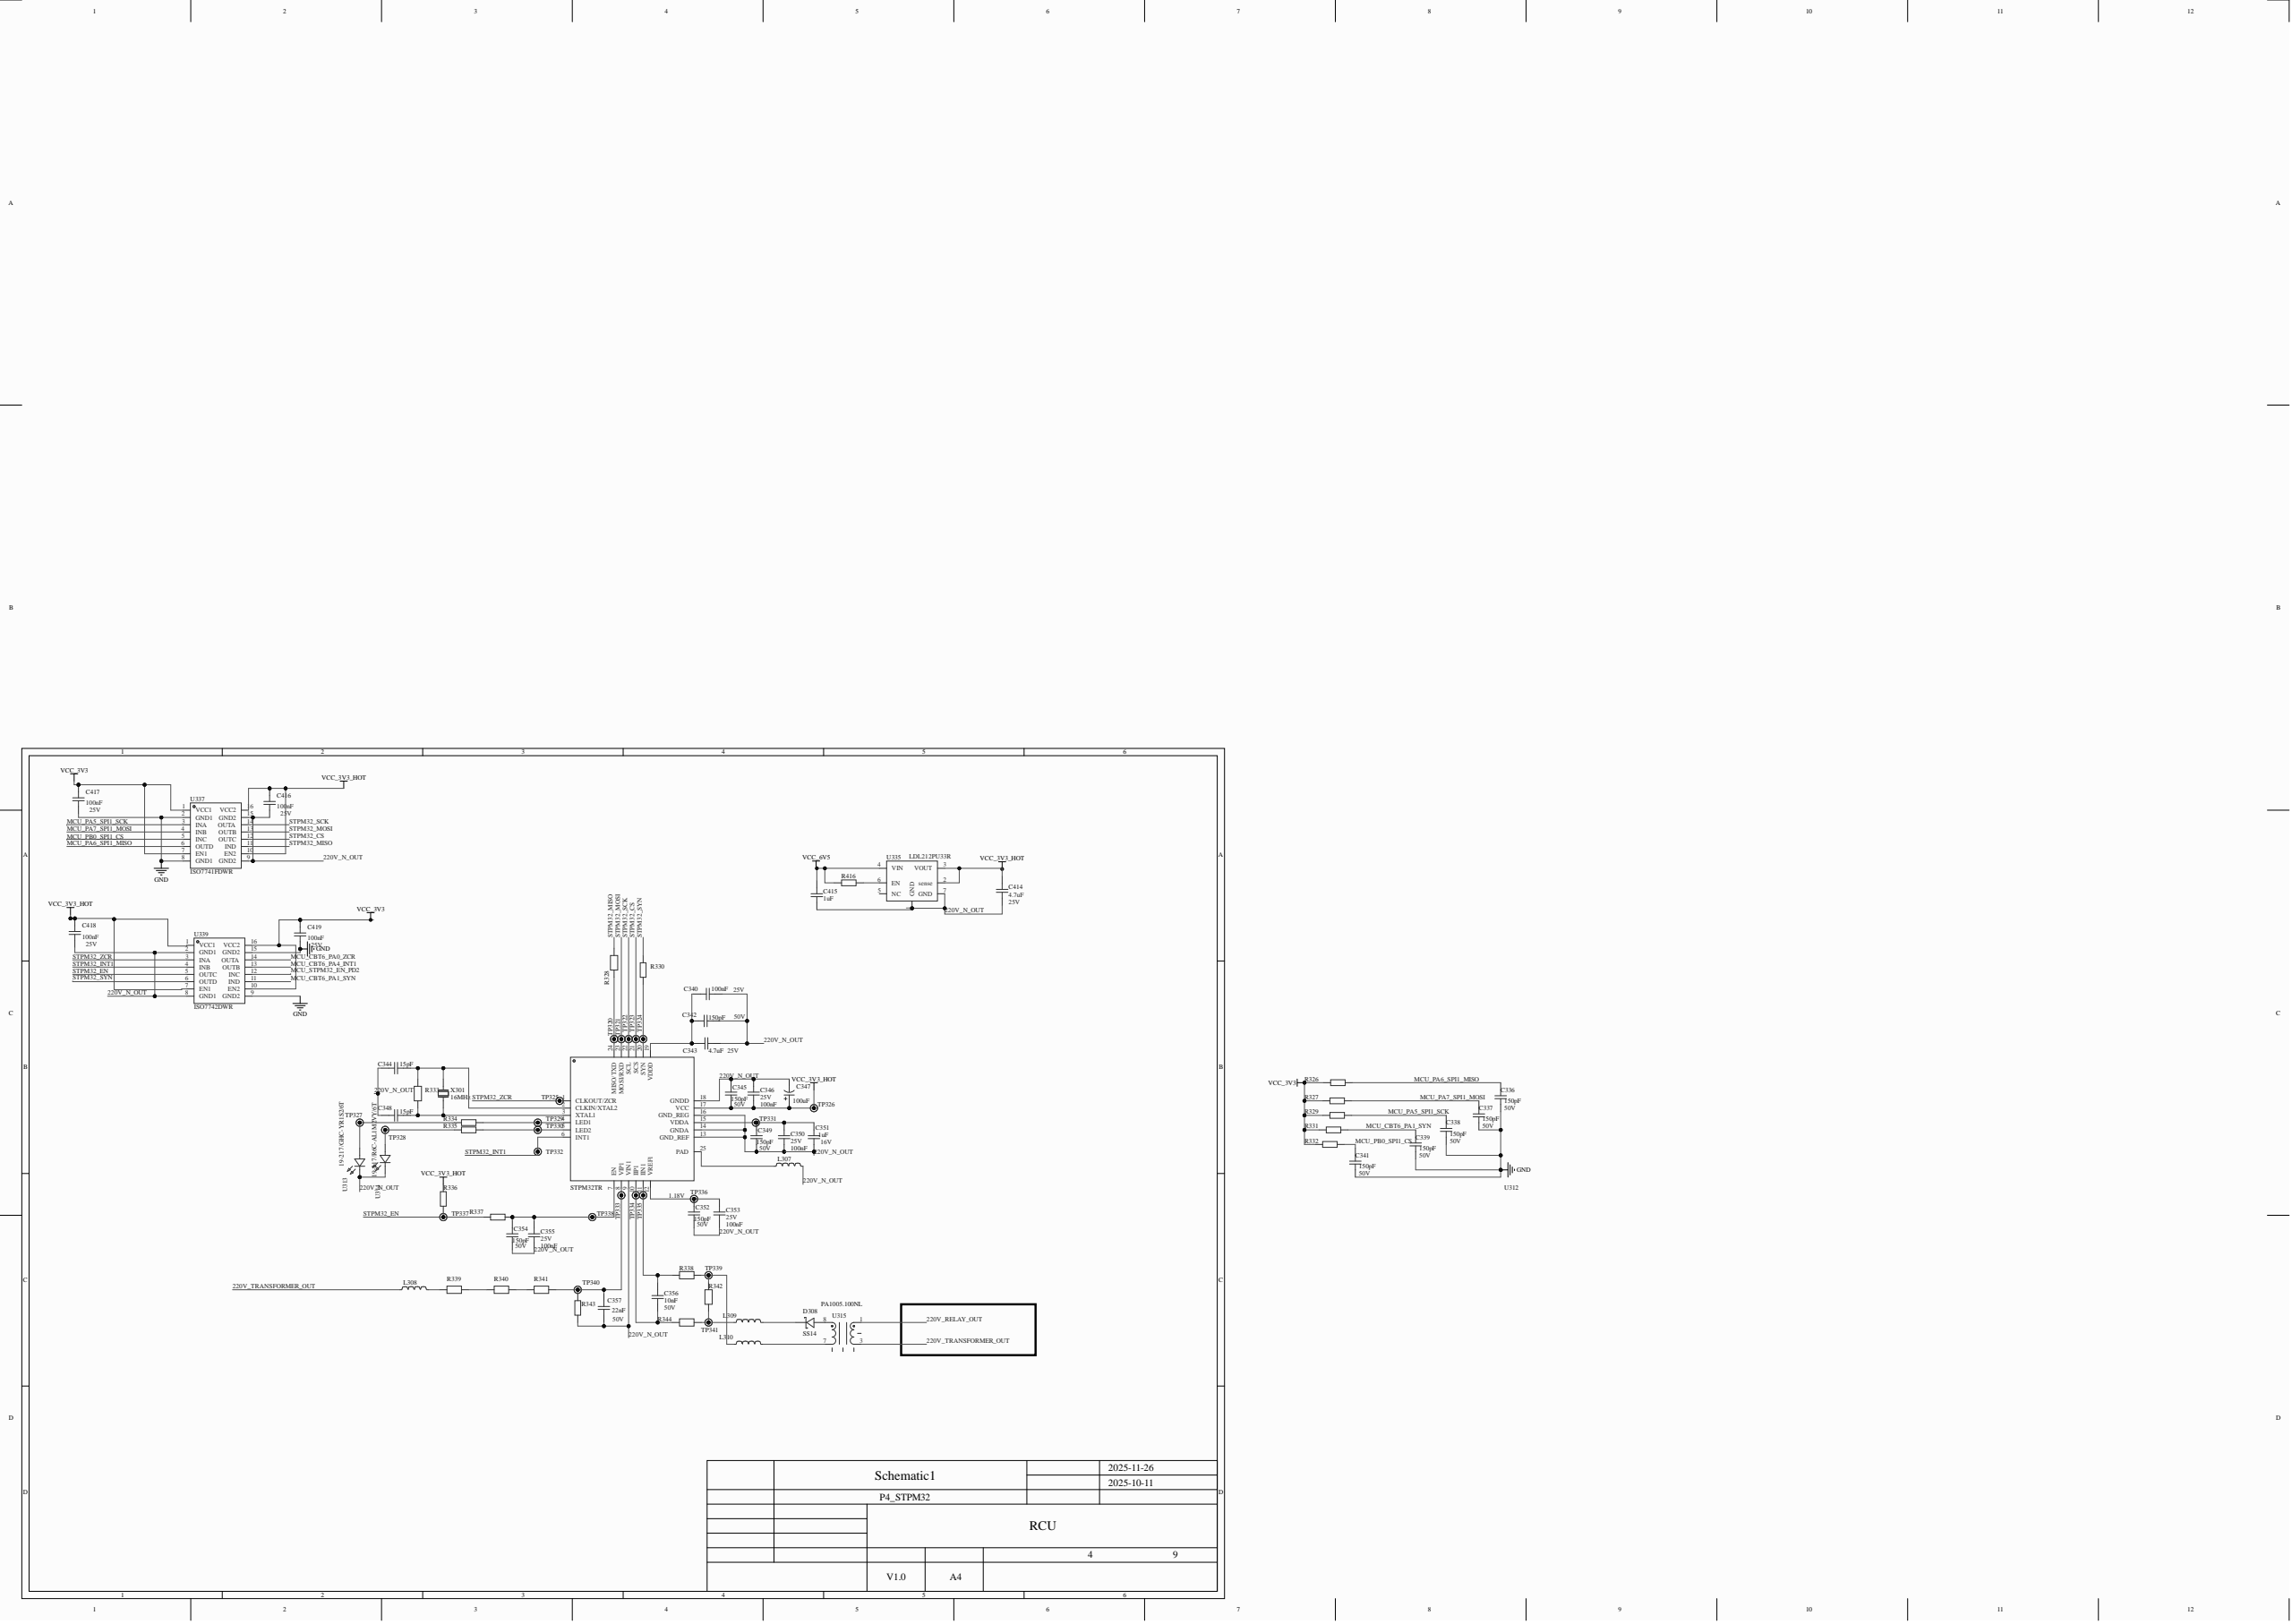Circuit board | Altium Designer | 424 parts | 202 nets | one sheet of the schematic
Parts on this sheet (reference | value | footprint):
C336 | 150pF | C0603
C337 | 150pF | C0603
C338 | 150pF | C0603
C339 | 150pF | C0603
C340 | 100nF | C0603
C341 | 150pF | C0603
C342 | 150pF | C0603
C343 | 4.7uF | C0603
C344 | 15pF | C0603
C345 | 150pF | C0603
C346 | 100nF | C0603
C347 | 100uF | CAP-SMD_BD6.3-L6.6-W6.6-LS7.3-FD-H7.7
C348 | 15pF | C0603
C349 | 150pF | C0603
C350 | 100nF | C0603
C351 | 1uF | C0603
C352 | 150pF | C0603
C353 | 100nF | C0603
C354 | 150pF | C0603
C355 | 100nF | C0603
C356 | 10nF | C0603
C357 | 22nF | C0805
C414 | 4.7uF | C0603
C415 | 1uF | C0603
C416 | 100nF | C0603
C417 | 100nF | C0603
C418 | 100nF | C0603
C419 | 100nF | C0603
D308 | SS14 | SMA_L4.3-W2.6-LS5.2-RD
L307 | L0805
L308 | L0805
L309 | L0805
L310 | L0805
R326 | R0603
R327 | R0603
R328 | R0603
R329 | R0603
R330 | R0603
R331 | R0603
R332 | R0603
R333 | R0603
R334 | R0603
R335 | R0603
R336 | R0603
R337 | R0603
R338 | R1206
R339 | R1206
R340 | R1206
R341 | R1206
R342 | R1206
R343 | R1206
R344 | R1206
R416 | R0603
TP320 | Test-Point-0.5mm
TP321 | Test-Point-0.5mm
TP322 | Test-Point-0.5mm
TP323 | Test-Point-0.5mm
TP324 | Test-Point-0.5mm
TP325 | Test-Point-0.5mm
TP326 | Test-Point-0.5mm
TP327 | Test-Point-0.5mm
TP328 | Test-Point-0.5mm
TP329 | Test-Point-0.5mm
TP330 | Test-Point-0.5mm
TP331 | Test-Point-0.5mm
TP332 | Test-Point-0.5mm
TP333 | Test-Point-0.5mm
TP334 | Test-Point-0.5mm
TP335 | Test-Point-0.5mm
TP336 | Test-Point-0.5mm
TP337 | Test-Point-0.5mm
TP338 | Test-Point-0.5mm
TP339 | Test-Point-0.5mm
TP340 | Test-Point-0.5mm
TP341 | Test-Point-0.5mm
U312 | STPM32TR | VQFN-24_L4.0-W4.0-P0.50-BL-EP2.3
U313 | 19-217/GHC-YR1S2/6T | LED0603-RD_GREEN
U314 | 19-217/R6C-AL1M2VY/6T | LED0603-R-FD
U315 | PA1005.100NL | SENSOR-TH_PA1005.100NL
U335 | LDL212PU33R | VSON-6_L3.0-W3.0-P0.95-TL-EP_TI_DRP
U337 | ISO7741FDWR | SOIC-16_L10.3-W7.5-P1.27-LS10.3-BL
U339 | ISO7742DWR | SOIC-16_L10.3-W7.5-P1.27-LS10.3-BL
X301 | 16MHz | CRYSTAL-SMD_2P-L5.0-W3.2
Nets of these parts (net: part-pin ...):
VCC_6V5: C415-2 R416-1 U335-4
VCC_3V3_HOT: C345-1 C346-1 C347-1 C414-2 C416-1 C418-1 R336-2 TP326-1 U335-2 U335-3 U337-10 U337-16 U339-1 U339-7 U312-17
VCC_3V3: C417-1 C419-1 R326-1 R327-1 R329-1 R331-1 R332-1 U337-1 U337-7 U339-10 U339-16
STPM32_ZCR: TP325-1 U339-3 U312-1
STPM32_SYN: R330-2 U339-6
STPM32_SCK: TP322-1 U337-14 U312-22
STPM32_MOSI: TP321-1 U337-13 U312-23
STPM32_MISO: R328-2 U337-11
STPM32_INT1: TP332-1 U339-4 U312-6
STPM32_EN: R336-1 R337-2 TP337-1 U339-5
STPM32_CS: TP323-1 U337-12 U312-21
NetR416_2: R416-2 U335-6
NetR340_2: R340-2 R341-2
NetR339_1: R339-1 R340-1
NetR335_2: R335-2 TP330-1 U312-5
NetR335_1: R335-1 TP328-1 U314-1
NetR334_2: R334-2 TP329-1 U312-4
NetR334_1: R334-1 TP327-1 U313-2
NetR330_1: R330-1 TP324-1 U312-20
NetR328_1: R328-1 TP320-1 U312-24
NetL310_2: L310-2 U315-7
NetL310_1: L310-1 R338-2 R342-2 TP339-1
NetL309_1: L309-1 R342-1 R344-2 TP341-1
NetL308_2: L308-2 R339-2
NetL307_1: L307-1 U312-25
NetD308_2: D308-2 U315-8
NetD308_1: D308-1 L309-2
NetC357_2: C357-2 R341-1 R343-2 TP333-1 TP340-1 U312-8
NetC356_2: C356-2 R338-1 TP335-1 U312-11
NetC356_1: C356-1 R344-1 TP334-1 U312-10
NetC354_2: C354-2 C355-2 R337-1 TP338-1 U312-7
NetC352_2: C352-2 C353-2 TP336-1 U312-12
NetC349_2: C349-2 C350-2 C351-2 TP331-1 U312-15
NetC348_2: C348-2 R333-1 X301-1 U312-3
NetC344_2: C344-2 R333-2 X301-2 U312-2
NetC340_1: C340-1 C342-1 C343-2 U312-19
MCU_STPM32_EN_PD2: U339-12
MCU_PB0_SPI1_CS: C341-1 R332-2 U337-5
MCU_PA7_SPI1_MOSI: C337-1 R327-2 U337-4
MCU_PA6_SPI1_MISO: C336-1 R326-2 U337-6
MCU_PA5_SPI1_SCK: C338-1 R329-2 U337-3
MCU_CBT6_PA4_INT1: U339-13
MCU_CBT6_PA1_SYN: C339-1 R331-2 U339-11
MCU_CBT6_PA0_ZCR: U339-14
GND: C336-2 C337-2 C338-2 C339-2 C341-2 C417-2 C419-2 U337-2 U337-8 U339-9 U339-15
220V_TRANSFORMER_OUT: L308-1 U315-3
220V_RELAY_OUT: U315-1
220V_N_OUT: C340-2 C342-2 C343-1 C344-1 C345-2 C346-2 C347-2 C348-1 C349-1 C350-1 C351-1 C352-1 C353-1 C354-1 C355-1 C357-1 C414-1 C415-1 C416-2 C418-2 L307-2 R343-1 U313-1 U314-2 U335-1 U335-7 U337-9 U337-15 U339-2 U339-8 U312-9 U312-13 U312-14 U312-16 U312-18